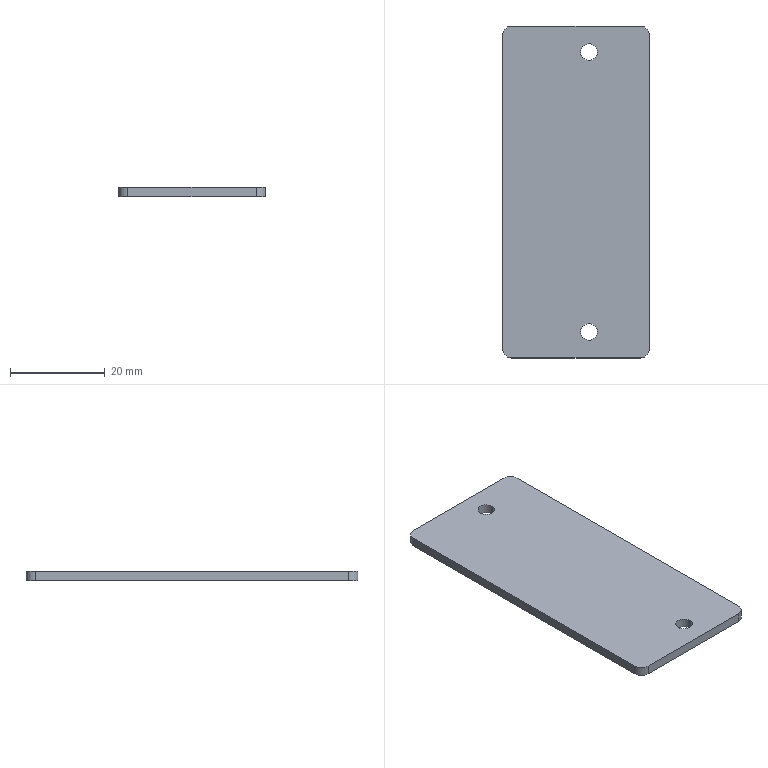Part | STEP file | 03-39 cutter pad plate | 1 solid | 14 faces | box 31 x 70 x 2 mm | volume 4295 mm3 | cylinder 8 | plane 6 | commonest cylinder face diameters 3.5 x4 4 x4
STEP:
#1=CARTESIAN_POINT('',(1.,-29.5,0.));
#2=VERTEX_POINT('',#1);
#3=CARTESIAN_POINT('',(4.5,-29.5,0.));
#4=VERTEX_POINT('',#3);
#5=CARTESIAN_POINT('',(2.75,-29.5,0.));
#6=DIRECTION('',(0.,0.,1.));
#7=DIRECTION('',(1.,0.,0.));
#8=AXIS2_PLACEMENT_3D('',#5,#6,#7);
#9=CIRCLE('',#8,1.75);
#10=EDGE_CURVE('',#2,#4,#9,.T.);
#11=ORIENTED_EDGE('',*,*,#10,.F.);
#12=CARTESIAN_POINT('',(1.,-29.5,2.));
#13=VERTEX_POINT('',#12);
#14=CARTESIAN_POINT('',(1.,-29.5,-8.));
#15=DIRECTION('',(0.,0.,1.));
#16=VECTOR('',#15,1000.);
#17=LINE('',#14,#16);
#18=EDGE_CURVE('',#2,#13,#17,.T.);
#19=ORIENTED_EDGE('',*,*,#18,.T.);
#20=CARTESIAN_POINT('',(4.5,-29.5,2.));
#21=VERTEX_POINT('',#20);
#22=CARTESIAN_POINT('',(2.75,-29.5,2.));
#23=DIRECTION('',(0.,0.,1.));
#24=DIRECTION('',(1.,0.,0.));
#25=AXIS2_PLACEMENT_3D('',#22,#23,#24);
#26=CIRCLE('',#25,1.75);
#27=EDGE_CURVE('',#13,#21,#26,.T.);
#28=ORIENTED_EDGE('',*,*,#27,.T.);
#29=CARTESIAN_POINT('',(4.5,-29.5,-8.));
#30=DIRECTION('',(0.,0.,1.));
#31=VECTOR('',#30,1000.);
#32=LINE('',#29,#31);
#33=EDGE_CURVE('',#4,#21,#32,.T.);
#34=ORIENTED_EDGE('',*,*,#33,.F.);
#35=EDGE_LOOP('',(#11,#19,#28,#34));
#36=FACE_OUTER_BOUND('',#35,.T.);
#37=CARTESIAN_POINT('',(2.75,-29.5,-8.));
#38=DIRECTION('',(0.,0.,1.));
#39=DIRECTION('',(1.,0.,0.));
#40=AXIS2_PLACEMENT_3D('',#37,#38,#39);
#41=CYLINDRICAL_SURFACE('',#40,1.75);
#42=ADVANCED_FACE('',(#36),#41,.F.);
#43=CARTESIAN_POINT('',(1.,29.5,0.));
#44=VERTEX_POINT('',#43);
#45=CARTESIAN_POINT('',(4.5,29.5,0.));
#46=VERTEX_POINT('',#45);
#47=CARTESIAN_POINT('',(2.75,29.5,0.));
#48=DIRECTION('',(0.,0.,1.));
#49=DIRECTION('',(1.,0.,0.));
#50=AXIS2_PLACEMENT_3D('',#47,#48,#49);
#51=CIRCLE('',#50,1.75);
#52=EDGE_CURVE('',#44,#46,#51,.T.);
#53=ORIENTED_EDGE('',*,*,#52,.F.);
#54=CARTESIAN_POINT('',(1.,29.5,2.));
#55=VERTEX_POINT('',#54);
#56=CARTESIAN_POINT('',(1.,29.5,-8.));
#57=DIRECTION('',(0.,0.,1.));
#58=VECTOR('',#57,1000.);
#59=LINE('',#56,#58);
#60=EDGE_CURVE('',#44,#55,#59,.T.);
#61=ORIENTED_EDGE('',*,*,#60,.T.);
#62=CARTESIAN_POINT('',(4.5,29.5,2.));
#63=VERTEX_POINT('',#62);
#64=CARTESIAN_POINT('',(2.75,29.5,2.));
#65=DIRECTION('',(0.,0.,1.));
#66=DIRECTION('',(1.,0.,0.));
#67=AXIS2_PLACEMENT_3D('',#64,#65,#66);
#68=CIRCLE('',#67,1.75);
#69=EDGE_CURVE('',#55,#63,#68,.T.);
#70=ORIENTED_EDGE('',*,*,#69,.T.);
#71=CARTESIAN_POINT('',(4.5,29.5,-8.));
#72=DIRECTION('',(0.,0.,1.));
#73=VECTOR('',#72,1000.);
#74=LINE('',#71,#73);
#75=EDGE_CURVE('',#46,#63,#74,.T.);
#76=ORIENTED_EDGE('',*,*,#75,.F.);
#77=EDGE_LOOP('',(#53,#61,#70,#76));
#78=FACE_OUTER_BOUND('',#77,.T.);
#79=CARTESIAN_POINT('',(2.75,29.5,-8.));
#80=DIRECTION('',(0.,0.,1.));
#81=DIRECTION('',(1.,0.,0.));
#82=AXIS2_PLACEMENT_3D('',#79,#80,#81);
#83=CYLINDRICAL_SURFACE('',#82,1.75);
#84=ADVANCED_FACE('',(#78),#83,.F.);
#85=CARTESIAN_POINT('',(15.5,-33.,0.));
#86=VERTEX_POINT('',#85);
#87=CARTESIAN_POINT('',(15.5,33.,0.));
#88=VERTEX_POINT('',#87);
#89=CARTESIAN_POINT('',(15.5,35.,0.));
#90=DIRECTION('',(0.,1.,0.));
#91=VECTOR('',#90,1000.);
#92=LINE('',#89,#91);
#93=EDGE_CURVE('',#86,#88,#92,.T.);
#94=ORIENTED_EDGE('',*,*,#93,.T.);
#95=CARTESIAN_POINT('',(15.5,33.,2.));
#96=VERTEX_POINT('',#95);
#97=CARTESIAN_POINT('',(15.5,33.,2.));
#98=DIRECTION('',(0.,0.,1.));
#99=VECTOR('',#98,1000.);
#100=LINE('',#97,#99);
#101=EDGE_CURVE('',#88,#96,#100,.T.);
#102=ORIENTED_EDGE('',*,*,#101,.T.);
#103=CARTESIAN_POINT('',(15.5,-33.,2.));
#104=VERTEX_POINT('',#103);
#105=CARTESIAN_POINT('',(15.5,35.,2.));
#106=DIRECTION('',(0.,1.,0.));
#107=VECTOR('',#106,1000.);
#108=LINE('',#105,#107);
#109=EDGE_CURVE('',#104,#96,#108,.T.);
#110=ORIENTED_EDGE('',*,*,#109,.F.);
#111=CARTESIAN_POINT('',(15.5,-33.,2.));
#112=DIRECTION('',(0.,0.,-1.));
#113=VECTOR('',#112,1000.);
#114=LINE('',#111,#113);
#115=EDGE_CURVE('',#104,#86,#114,.T.);
#116=ORIENTED_EDGE('',*,*,#115,.T.);
#117=EDGE_LOOP('',(#94,#102,#110,#116));
#118=FACE_OUTER_BOUND('',#117,.T.);
#119=CARTESIAN_POINT('',(15.5,35.,2.));
#120=DIRECTION('',(-1.,0.,0.));
#121=DIRECTION('',(0.,-1.,0.));
#122=AXIS2_PLACEMENT_3D('',#119,#120,#121);
#123=PLANE('',#122);
#124=ADVANCED_FACE('',(#118),#123,.F.);
#125=CARTESIAN_POINT('',(13.5,35.,0.));
#126=VERTEX_POINT('',#125);
#127=CARTESIAN_POINT('',(-13.5,35.,0.));
#128=VERTEX_POINT('',#127);
#129=CARTESIAN_POINT('',(-15.5,35.,0.));
#130=DIRECTION('',(-1.,0.,0.));
#131=VECTOR('',#130,1000.);
#132=LINE('',#129,#131);
#133=EDGE_CURVE('',#126,#128,#132,.T.);
#134=ORIENTED_EDGE('',*,*,#133,.T.);
#135=CARTESIAN_POINT('',(-13.5,35.,2.));
#136=VERTEX_POINT('',#135);
#137=CARTESIAN_POINT('',(-13.5,35.,2.));
#138=DIRECTION('',(0.,0.,1.));
#139=VECTOR('',#138,1000.);
#140=LINE('',#137,#139);
#141=EDGE_CURVE('',#128,#136,#140,.T.);
#142=ORIENTED_EDGE('',*,*,#141,.T.);
#143=CARTESIAN_POINT('',(13.5,35.,2.));
#144=VERTEX_POINT('',#143);
#145=CARTESIAN_POINT('',(-15.5,35.,2.));
#146=DIRECTION('',(-1.,0.,0.));
#147=VECTOR('',#146,1000.);
#148=LINE('',#145,#147);
#149=EDGE_CURVE('',#144,#136,#148,.T.);
#150=ORIENTED_EDGE('',*,*,#149,.F.);
#151=CARTESIAN_POINT('',(13.5,35.,2.));
#152=DIRECTION('',(0.,0.,-1.));
#153=VECTOR('',#152,1000.);
#154=LINE('',#151,#153);
#155=EDGE_CURVE('',#144,#126,#154,.T.);
#156=ORIENTED_EDGE('',*,*,#155,.T.);
#157=EDGE_LOOP('',(#134,#142,#150,#156));
#158=FACE_OUTER_BOUND('',#157,.T.);
#159=CARTESIAN_POINT('',(-15.5,35.,2.));
#160=DIRECTION('',(0.,-1.,0.));
#161=DIRECTION('',(0.,0.,-1.));
#162=AXIS2_PLACEMENT_3D('',#159,#160,#161);
#163=PLANE('',#162);
#164=ADVANCED_FACE('',(#158),#163,.F.);
#165=CARTESIAN_POINT('',(-15.5,33.,2.));
#166=VERTEX_POINT('',#165);
#167=CARTESIAN_POINT('',(-15.5,-33.,2.));
#168=VERTEX_POINT('',#167);
#169=CARTESIAN_POINT('',(-15.5,35.,2.));
#170=DIRECTION('',(0.,-1.,0.));
#171=VECTOR('',#170,1000.);
#172=LINE('',#169,#171);
#173=EDGE_CURVE('',#166,#168,#172,.T.);
#174=ORIENTED_EDGE('',*,*,#173,.F.);
#175=CARTESIAN_POINT('',(-15.5,33.,0.));
#176=VERTEX_POINT('',#175);
#177=CARTESIAN_POINT('',(-15.5,33.,2.));
#178=DIRECTION('',(0.,0.,-1.));
#179=VECTOR('',#178,1000.);
#180=LINE('',#177,#179);
#181=EDGE_CURVE('',#166,#176,#180,.T.);
#182=ORIENTED_EDGE('',*,*,#181,.T.);
#183=CARTESIAN_POINT('',(-15.5,-33.,0.));
#184=VERTEX_POINT('',#183);
#185=CARTESIAN_POINT('',(-15.5,35.,0.));
#186=DIRECTION('',(0.,-1.,0.));
#187=VECTOR('',#186,1000.);
#188=LINE('',#185,#187);
#189=EDGE_CURVE('',#176,#184,#188,.T.);
#190=ORIENTED_EDGE('',*,*,#189,.T.);
#191=CARTESIAN_POINT('',(-15.5,-33.,2.));
#192=DIRECTION('',(0.,0.,1.));
#193=VECTOR('',#192,1000.);
#194=LINE('',#191,#193);
#195=EDGE_CURVE('',#184,#168,#194,.T.);
#196=ORIENTED_EDGE('',*,*,#195,.T.);
#197=EDGE_LOOP('',(#174,#182,#190,#196));
#198=FACE_OUTER_BOUND('',#197,.T.);
#199=CARTESIAN_POINT('',(-15.5,35.,2.));
#200=DIRECTION('',(1.,0.,0.));
#201=DIRECTION('',(0.,1.,0.));
#202=AXIS2_PLACEMENT_3D('',#199,#200,#201);
#203=PLANE('',#202);
#204=ADVANCED_FACE('',(#198),#203,.F.);
#205=CARTESIAN_POINT('',(-13.5,-35.,0.));
#206=VERTEX_POINT('',#205);
#207=CARTESIAN_POINT('',(13.5,-35.,0.));
#208=VERTEX_POINT('',#207);
#209=CARTESIAN_POINT('',(-15.5,-35.,0.));
#210=DIRECTION('',(1.,0.,0.));
#211=VECTOR('',#210,1000.);
#212=LINE('',#209,#211);
#213=EDGE_CURVE('',#206,#208,#212,.T.);
#214=ORIENTED_EDGE('',*,*,#213,.T.);
#215=CARTESIAN_POINT('',(13.5,-35.,2.));
#216=VERTEX_POINT('',#215);
#217=CARTESIAN_POINT('',(13.5,-35.,2.));
#218=DIRECTION('',(0.,0.,1.));
#219=VECTOR('',#218,1000.);
#220=LINE('',#217,#219);
#221=EDGE_CURVE('',#208,#216,#220,.T.);
#222=ORIENTED_EDGE('',*,*,#221,.T.);
#223=CARTESIAN_POINT('',(-13.5,-35.,2.));
#224=VERTEX_POINT('',#223);
#225=CARTESIAN_POINT('',(-15.5,-35.,2.));
#226=DIRECTION('',(1.,0.,0.));
#227=VECTOR('',#226,1000.);
#228=LINE('',#225,#227);
#229=EDGE_CURVE('',#224,#216,#228,.T.);
#230=ORIENTED_EDGE('',*,*,#229,.F.);
#231=CARTESIAN_POINT('',(-13.5,-35.,2.));
#232=DIRECTION('',(0.,0.,-1.));
#233=VECTOR('',#232,1000.);
#234=LINE('',#231,#233);
#235=EDGE_CURVE('',#224,#206,#234,.T.);
#236=ORIENTED_EDGE('',*,*,#235,.T.);
#237=EDGE_LOOP('',(#214,#222,#230,#236));
#238=FACE_OUTER_BOUND('',#237,.T.);
#239=CARTESIAN_POINT('',(-15.5,-35.,2.));
#240=DIRECTION('',(0.,1.,0.));
#241=DIRECTION('',(0.,0.,1.));
#242=AXIS2_PLACEMENT_3D('',#239,#240,#241);
#243=PLANE('',#242);
#244=ADVANCED_FACE('',(#238),#243,.F.);
#245=CARTESIAN_POINT('',(2.75,-29.5,2.));
#246=DIRECTION('',(0.,0.,1.));
#247=DIRECTION('',(1.,0.,0.));
#248=AXIS2_PLACEMENT_3D('',#245,#246,#247);
#249=CIRCLE('',#248,1.75);
#250=EDGE_CURVE('',#21,#13,#249,.T.);
#251=ORIENTED_EDGE('',*,*,#250,.F.);
#252=ORIENTED_EDGE('',*,*,#27,.F.);
#253=EDGE_LOOP('',(#251,#252));
#254=FACE_BOUND('',#253,.T.);
#255=CARTESIAN_POINT('',(2.75,29.5,2.));
#256=DIRECTION('',(0.,0.,1.));
#257=DIRECTION('',(1.,0.,0.));
#258=AXIS2_PLACEMENT_3D('',#255,#256,#257);
#259=CIRCLE('',#258,1.75);
#260=EDGE_CURVE('',#63,#55,#259,.T.);
#261=ORIENTED_EDGE('',*,*,#260,.F.);
#262=ORIENTED_EDGE('',*,*,#69,.F.);
#263=EDGE_LOOP('',(#261,#262));
#264=FACE_BOUND('',#263,.T.);
#265=ORIENTED_EDGE('',*,*,#149,.T.);
#266=CARTESIAN_POINT('',(-13.5,33.,2.));
#267=DIRECTION('',(0.,0.,1.));
#268=DIRECTION('',(1.,0.,0.));
#269=AXIS2_PLACEMENT_3D('',#266,#267,#268);
#270=CIRCLE('',#269,2.);
#271=EDGE_CURVE('',#136,#166,#270,.T.);
#272=ORIENTED_EDGE('',*,*,#271,.T.);
#273=ORIENTED_EDGE('',*,*,#173,.T.);
#274=CARTESIAN_POINT('',(-13.5,-33.,2.));
#275=DIRECTION('',(0.,0.,1.));
#276=DIRECTION('',(1.,0.,0.));
#277=AXIS2_PLACEMENT_3D('',#274,#275,#276);
#278=CIRCLE('',#277,2.);
#279=EDGE_CURVE('',#168,#224,#278,.T.);
#280=ORIENTED_EDGE('',*,*,#279,.T.);
#281=ORIENTED_EDGE('',*,*,#229,.T.);
#282=CARTESIAN_POINT('',(13.5,-33.,2.));
#283=DIRECTION('',(0.,0.,1.));
#284=DIRECTION('',(1.,0.,0.));
#285=AXIS2_PLACEMENT_3D('',#282,#283,#284);
#286=CIRCLE('',#285,2.);
#287=EDGE_CURVE('',#216,#104,#286,.T.);
#288=ORIENTED_EDGE('',*,*,#287,.T.);
#289=ORIENTED_EDGE('',*,*,#109,.T.);
#290=CARTESIAN_POINT('',(13.5,33.,2.));
#291=DIRECTION('',(0.,0.,1.));
#292=DIRECTION('',(1.,0.,0.));
#293=AXIS2_PLACEMENT_3D('',#290,#291,#292);
#294=CIRCLE('',#293,2.);
#295=EDGE_CURVE('',#96,#144,#294,.T.);
#296=ORIENTED_EDGE('',*,*,#295,.T.);
#297=EDGE_LOOP('',(#265,#272,#273,#280,#281,#288,#289,#296));
#298=FACE_OUTER_BOUND('',#297,.T.);
#299=CARTESIAN_POINT('',(15.5,-35.,2.));
#300=DIRECTION('',(0.,0.,1.));
#301=DIRECTION('',(1.,0.,0.));
#302=AXIS2_PLACEMENT_3D('',#299,#300,#301);
#303=PLANE('',#302);
#304=ADVANCED_FACE('',(#254,#264,#298),#303,.T.);
#305=CARTESIAN_POINT('',(2.75,-29.5,0.));
#306=DIRECTION('',(0.,0.,1.));
#307=DIRECTION('',(1.,0.,0.));
#308=AXIS2_PLACEMENT_3D('',#305,#306,#307);
#309=CIRCLE('',#308,1.75);
#310=EDGE_CURVE('',#4,#2,#309,.T.);
#311=ORIENTED_EDGE('',*,*,#310,.T.);
#312=ORIENTED_EDGE('',*,*,#10,.T.);
#313=EDGE_LOOP('',(#311,#312));
#314=FACE_BOUND('',#313,.T.);
#315=CARTESIAN_POINT('',(2.75,29.5,0.));
#316=DIRECTION('',(0.,0.,1.));
#317=DIRECTION('',(1.,0.,0.));
#318=AXIS2_PLACEMENT_3D('',#315,#316,#317);
#319=CIRCLE('',#318,1.75);
#320=EDGE_CURVE('',#46,#44,#319,.T.);
#321=ORIENTED_EDGE('',*,*,#320,.T.);
#322=ORIENTED_EDGE('',*,*,#52,.T.);
#323=EDGE_LOOP('',(#321,#322));
#324=FACE_BOUND('',#323,.T.);
#325=ORIENTED_EDGE('',*,*,#189,.F.);
#326=CARTESIAN_POINT('',(-13.5,33.,0.));
#327=DIRECTION('',(0.,0.,-1.));
#328=DIRECTION('',(1.,0.,0.));
#329=AXIS2_PLACEMENT_3D('',#326,#327,#328);
#330=CIRCLE('',#329,2.);
#331=EDGE_CURVE('',#176,#128,#330,.T.);
#332=ORIENTED_EDGE('',*,*,#331,.T.);
#333=ORIENTED_EDGE('',*,*,#133,.F.);
#334=CARTESIAN_POINT('',(13.5,33.,0.));
#335=DIRECTION('',(0.,0.,-1.));
#336=DIRECTION('',(1.,0.,0.));
#337=AXIS2_PLACEMENT_3D('',#334,#335,#336);
#338=CIRCLE('',#337,2.);
#339=EDGE_CURVE('',#126,#88,#338,.T.);
#340=ORIENTED_EDGE('',*,*,#339,.T.);
#341=ORIENTED_EDGE('',*,*,#93,.F.);
#342=CARTESIAN_POINT('',(13.5,-33.,0.));
#343=DIRECTION('',(0.,0.,-1.));
#344=DIRECTION('',(1.,0.,0.));
#345=AXIS2_PLACEMENT_3D('',#342,#343,#344);
#346=CIRCLE('',#345,2.);
#347=EDGE_CURVE('',#86,#208,#346,.T.);
#348=ORIENTED_EDGE('',*,*,#347,.T.);
#349=ORIENTED_EDGE('',*,*,#213,.F.);
#350=CARTESIAN_POINT('',(-13.5,-33.,0.));
#351=DIRECTION('',(0.,0.,-1.));
#352=DIRECTION('',(1.,0.,0.));
#353=AXIS2_PLACEMENT_3D('',#350,#351,#352);
#354=CIRCLE('',#353,2.);
#355=EDGE_CURVE('',#206,#184,#354,.T.);
#356=ORIENTED_EDGE('',*,*,#355,.T.);
#357=EDGE_LOOP('',(#325,#332,#333,#340,#341,#348,#349,#356));
#358=FACE_OUTER_BOUND('',#357,.T.);
#359=CARTESIAN_POINT('',(15.5,-35.,0.));
#360=DIRECTION('',(0.,0.,1.));
#361=DIRECTION('',(1.,0.,0.));
#362=AXIS2_PLACEMENT_3D('',#359,#360,#361);
#363=PLANE('',#362);
#364=ADVANCED_FACE('',(#314,#324,#358),#363,.F.);
#365=ORIENTED_EDGE('',*,*,#60,.F.);
#366=ORIENTED_EDGE('',*,*,#320,.F.);
#367=ORIENTED_EDGE('',*,*,#75,.T.);
#368=ORIENTED_EDGE('',*,*,#260,.T.);
#369=EDGE_LOOP('',(#365,#366,#367,#368));
#370=FACE_OUTER_BOUND('',#369,.T.);
#371=CARTESIAN_POINT('',(2.75,29.5,-8.));
#372=DIRECTION('',(0.,0.,1.));
#373=DIRECTION('',(1.,0.,0.));
#374=AXIS2_PLACEMENT_3D('',#371,#372,#373);
#375=CYLINDRICAL_SURFACE('',#374,1.75);
#376=ADVANCED_FACE('',(#370),#375,.F.);
#377=ORIENTED_EDGE('',*,*,#18,.F.);
#378=ORIENTED_EDGE('',*,*,#310,.F.);
#379=ORIENTED_EDGE('',*,*,#33,.T.);
#380=ORIENTED_EDGE('',*,*,#250,.T.);
#381=EDGE_LOOP('',(#377,#378,#379,#380));
#382=FACE_OUTER_BOUND('',#381,.T.);
#383=CARTESIAN_POINT('',(2.75,-29.5,-8.));
#384=DIRECTION('',(0.,0.,1.));
#385=DIRECTION('',(1.,0.,0.));
#386=AXIS2_PLACEMENT_3D('',#383,#384,#385);
#387=CYLINDRICAL_SURFACE('',#386,1.75);
#388=ADVANCED_FACE('',(#382),#387,.F.);
#389=ORIENTED_EDGE('',*,*,#271,.F.);
#390=ORIENTED_EDGE('',*,*,#141,.F.);
#391=ORIENTED_EDGE('',*,*,#331,.F.);
#392=ORIENTED_EDGE('',*,*,#181,.F.);
#393=EDGE_LOOP('',(#389,#390,#391,#392));
#394=FACE_OUTER_BOUND('',#393,.T.);
#395=CARTESIAN_POINT('',(-13.5,33.,2.));
#396=DIRECTION('',(0.,0.,-1.));
#397=DIRECTION('',(-1.,0.,0.));
#398=AXIS2_PLACEMENT_3D('',#395,#396,#397);
#399=CYLINDRICAL_SURFACE('',#398,2.);
#400=ADVANCED_FACE('',(#394),#399,.T.);
#401=ORIENTED_EDGE('',*,*,#295,.F.);
#402=ORIENTED_EDGE('',*,*,#101,.F.);
#403=ORIENTED_EDGE('',*,*,#339,.F.);
#404=ORIENTED_EDGE('',*,*,#155,.F.);
#405=EDGE_LOOP('',(#401,#402,#403,#404));
#406=FACE_OUTER_BOUND('',#405,.T.);
#407=CARTESIAN_POINT('',(13.5,33.,2.));
#408=DIRECTION('',(0.,0.,-1.));
#409=DIRECTION('',(-1.,0.,0.));
#410=AXIS2_PLACEMENT_3D('',#407,#408,#409);
#411=CYLINDRICAL_SURFACE('',#410,2.);
#412=ADVANCED_FACE('',(#406),#411,.T.);
#413=ORIENTED_EDGE('',*,*,#287,.F.);
#414=ORIENTED_EDGE('',*,*,#221,.F.);
#415=ORIENTED_EDGE('',*,*,#347,.F.);
#416=ORIENTED_EDGE('',*,*,#115,.F.);
#417=EDGE_LOOP('',(#413,#414,#415,#416));
#418=FACE_OUTER_BOUND('',#417,.T.);
#419=CARTESIAN_POINT('',(13.5,-33.,2.));
#420=DIRECTION('',(0.,0.,-1.));
#421=DIRECTION('',(-1.,0.,0.));
#422=AXIS2_PLACEMENT_3D('',#419,#420,#421);
#423=CYLINDRICAL_SURFACE('',#422,2.);
#424=ADVANCED_FACE('',(#418),#423,.T.);
#425=ORIENTED_EDGE('',*,*,#279,.F.);
#426=ORIENTED_EDGE('',*,*,#195,.F.);
#427=ORIENTED_EDGE('',*,*,#355,.F.);
#428=ORIENTED_EDGE('',*,*,#235,.F.);
#429=EDGE_LOOP('',(#425,#426,#427,#428));
#430=FACE_OUTER_BOUND('',#429,.T.);
#431=CARTESIAN_POINT('',(-13.5,-33.,2.));
#432=DIRECTION('',(0.,0.,-1.));
#433=DIRECTION('',(-1.,0.,0.));
#434=AXIS2_PLACEMENT_3D('',#431,#432,#433);
#435=CYLINDRICAL_SURFACE('',#434,2.);
#436=ADVANCED_FACE('',(#430),#435,.T.);
#437=CLOSED_SHELL('',(#42,#84,#124,#164,#204,#244,#304,#364,#376,#388,#400,#412,#424,#436));
#438=MANIFOLD_SOLID_BREP('',#437);
#439=CARTESIAN_POINT('',(0.,0.,0.));
#440=DIRECTION('',(0.,0.,1.));
#441=DIRECTION('',(1.,0.,0.));
#442=AXIS2_PLACEMENT_3D('',#439,#440,#441);
#443=(LENGTH_UNIT()NAMED_UNIT(*)SI_UNIT(.MILLI.,.METRE.));
#444=UNCERTAINTY_MEASURE_WITH_UNIT(LENGTH_MEASURE(0.00001),#443,'','');
#445=(NAMED_UNIT(*)PLANE_ANGLE_UNIT()SI_UNIT($,.RADIAN.));
#446=(NAMED_UNIT(*)SI_UNIT($,.STERADIAN.)SOLID_ANGLE_UNIT());
#447=(GEOMETRIC_REPRESENTATION_CONTEXT(3)GLOBAL_UNCERTAINTY_ASSIGNED_CONTEXT((#444))GLOBAL_UNIT_ASSIGNED_CONTEXT((#443,#445,#446))REPRESENTATION_CONTEXT('',''));
#448=ADVANCED_BREP_SHAPE_REPRESENTATION('',(#438,#442),#447);